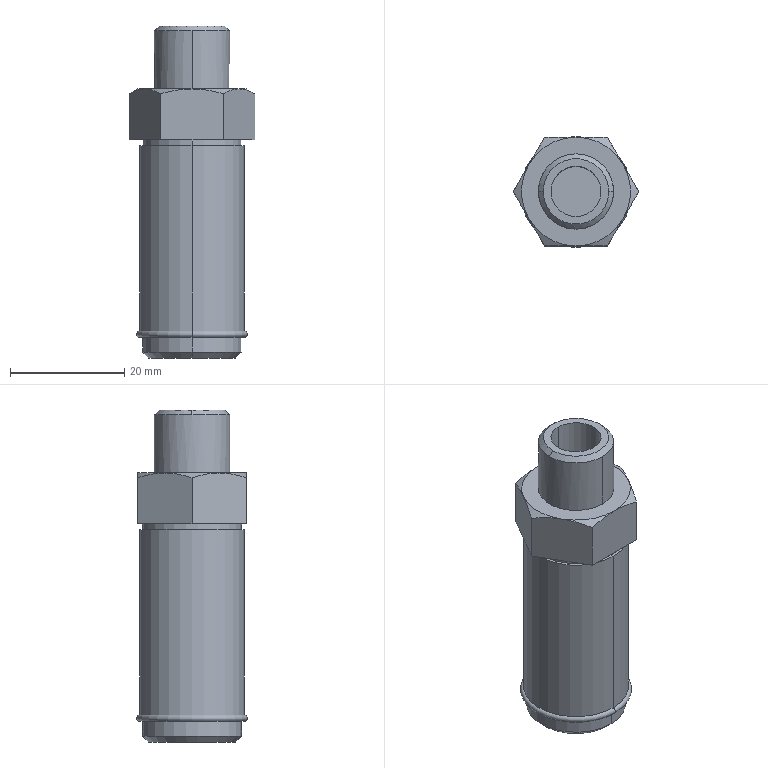Part | STEP file | _HSV08 Body.... | 1 solid | 40 faces | box 21.939 x 19.4 x 58 mm | volume 11796 mm3 | plane 14 | cylinder 12 | cone 12 | torus 2 | commonest cylinder face diameters 17.3 x4 8.771 x2 11.445 x2 13.157 x2 18.3 x2
STEP:
#1=CARTESIAN_POINT('',(0.,-9.15,1.1));
#2=VERTEX_POINT('',#1);
#3=CARTESIAN_POINT('',(0.,9.15,1.1));
#4=VERTEX_POINT('',#3);
#5=CARTESIAN_POINT('',(0.,0.,1.1));
#6=DIRECTION('',(0.,0.,1.));
#7=DIRECTION('',(0.,-1.,0.));
#8=AXIS2_PLACEMENT_3D('',#5,#6,#7);
#9=CIRCLE('',#8,9.15);
#10=EDGE_CURVE('',#2,#4,#9,.T.);
#11=ORIENTED_EDGE('',*,*,#10,.T.);
#12=CARTESIAN_POINT('',(0.,9.15,33.5));
#13=VERTEX_POINT('',#12);
#14=CARTESIAN_POINT('',(0.,9.15,-3.6));
#15=DIRECTION('',(0.,0.,1.));
#16=VECTOR('',#15,1000.);
#17=LINE('',#14,#16);
#18=EDGE_CURVE('',#4,#13,#17,.T.);
#19=ORIENTED_EDGE('',*,*,#18,.T.);
#20=CARTESIAN_POINT('',(0.,-9.15,33.5));
#21=VERTEX_POINT('',#20);
#22=CARTESIAN_POINT('',(0.,0.,33.5));
#23=DIRECTION('',(0.,0.,-1.));
#24=DIRECTION('',(0.,-1.,0.));
#25=AXIS2_PLACEMENT_3D('',#22,#23,#24);
#26=CIRCLE('',#25,9.15);
#27=EDGE_CURVE('',#13,#21,#26,.T.);
#28=ORIENTED_EDGE('',*,*,#27,.T.);
#29=CARTESIAN_POINT('',(0.,-9.15,-3.6));
#30=DIRECTION('',(0.,0.,1.));
#31=VECTOR('',#30,1000.);
#32=LINE('',#29,#31);
#33=EDGE_CURVE('',#2,#21,#32,.T.);
#34=ORIENTED_EDGE('',*,*,#33,.F.);
#35=EDGE_LOOP('',(#11,#19,#28,#34));
#36=FACE_OUTER_BOUND('',#35,.T.);
#37=CARTESIAN_POINT('',(0.,0.,-3.6));
#38=DIRECTION('',(0.,0.,1.));
#39=DIRECTION('',(0.,-1.,0.));
#40=AXIS2_PLACEMENT_3D('',#37,#38,#39);
#41=CYLINDRICAL_SURFACE('',#40,9.15);
#42=ADVANCED_FACE('',(#36),#41,.T.);
#43=ORIENTED_EDGE('',*,*,#10,.F.);
#44=CARTESIAN_POINT('',(0.,-9.15,0.));
#45=VERTEX_POINT('',#44);
#46=CARTESIAN_POINT('',(0.,-9.15,0.55));
#47=DIRECTION('',(1.,0.,0.));
#48=DIRECTION('',(0.,1.,0.));
#49=AXIS2_PLACEMENT_3D('',#46,#47,#48);
#50=CIRCLE('',#49,0.55);
#51=EDGE_CURVE('',#2,#45,#50,.T.);
#52=ORIENTED_EDGE('',*,*,#51,.T.);
#53=CARTESIAN_POINT('',(0.,9.15,0.));
#54=VERTEX_POINT('',#53);
#55=CARTESIAN_POINT('',(0.,0.,0.));
#56=DIRECTION('',(0.,0.,1.));
#57=DIRECTION('',(0.,1.,0.));
#58=AXIS2_PLACEMENT_3D('',#55,#56,#57);
#59=CIRCLE('',#58,9.15);
#60=EDGE_CURVE('',#45,#54,#59,.T.);
#61=ORIENTED_EDGE('',*,*,#60,.T.);
#62=CARTESIAN_POINT('',(0.,9.15,0.55));
#63=DIRECTION('',(-1.,0.,0.));
#64=DIRECTION('',(0.,0.,1.));
#65=AXIS2_PLACEMENT_3D('',#62,#63,#64);
#66=CIRCLE('',#65,0.55);
#67=EDGE_CURVE('',#4,#54,#66,.T.);
#68=ORIENTED_EDGE('',*,*,#67,.F.);
#69=EDGE_LOOP('',(#43,#52,#61,#68));
#70=FACE_OUTER_BOUND('',#69,.T.);
#71=CARTESIAN_POINT('',(0.,0.,0.55));
#72=DIRECTION('',(0.,0.,-1.));
#73=DIRECTION('',(0.,1.,0.));
#74=AXIS2_PLACEMENT_3D('',#71,#72,#73);
#75=TOROIDAL_SURFACE('',#74,9.15,0.55);
#76=ADVANCED_FACE('',(#70),#75,.T.);
#77=CARTESIAN_POINT('',(0.,-8.65,33.5));
#78=VERTEX_POINT('',#77);
#79=CARTESIAN_POINT('',(0.,8.65,33.5));
#80=VERTEX_POINT('',#79);
#81=CARTESIAN_POINT('',(0.,0.,33.5));
#82=DIRECTION('',(0.,0.,1.));
#83=DIRECTION('',(0.,-1.,0.));
#84=AXIS2_PLACEMENT_3D('',#81,#82,#83);
#85=CIRCLE('',#84,8.65);
#86=EDGE_CURVE('',#78,#80,#85,.T.);
#87=ORIENTED_EDGE('',*,*,#86,.T.);
#88=CARTESIAN_POINT('',(0.,8.65,34.5));
#89=VERTEX_POINT('',#88);
#90=CARTESIAN_POINT('',(0.,8.65,-3.6));
#91=DIRECTION('',(0.,0.,1.));
#92=VECTOR('',#91,1000.);
#93=LINE('',#90,#92);
#94=EDGE_CURVE('',#80,#89,#93,.T.);
#95=ORIENTED_EDGE('',*,*,#94,.T.);
#96=CARTESIAN_POINT('',(0.,-8.65,34.5));
#97=VERTEX_POINT('',#96);
#98=CARTESIAN_POINT('',(0.,0.,34.5));
#99=DIRECTION('',(0.,0.,-1.));
#100=DIRECTION('',(0.,-1.,0.));
#101=AXIS2_PLACEMENT_3D('',#98,#99,#100);
#102=CIRCLE('',#101,8.65);
#103=EDGE_CURVE('',#89,#97,#102,.T.);
#104=ORIENTED_EDGE('',*,*,#103,.T.);
#105=CARTESIAN_POINT('',(0.,-8.65,-3.6));
#106=DIRECTION('',(0.,0.,1.));
#107=VECTOR('',#106,1000.);
#108=LINE('',#105,#107);
#109=EDGE_CURVE('',#78,#97,#108,.T.);
#110=ORIENTED_EDGE('',*,*,#109,.F.);
#111=EDGE_LOOP('',(#87,#95,#104,#110));
#112=FACE_OUTER_BOUND('',#111,.T.);
#113=CARTESIAN_POINT('',(0.,0.,-3.6));
#114=DIRECTION('',(0.,0.,1.));
#115=DIRECTION('',(0.,-1.,0.));
#116=AXIS2_PLACEMENT_3D('',#113,#114,#115);
#117=CYLINDRICAL_SURFACE('',#116,8.65);
#118=ADVANCED_FACE('',(#112),#117,.T.);
#119=CARTESIAN_POINT('',(0.,-8.65,-2.6));
#120=VERTEX_POINT('',#119);
#121=CARTESIAN_POINT('',(0.,8.65,-2.6));
#122=VERTEX_POINT('',#121);
#123=CARTESIAN_POINT('',(0.,0.,-2.6));
#124=DIRECTION('',(0.,0.,1.));
#125=DIRECTION('',(0.,-1.,0.));
#126=AXIS2_PLACEMENT_3D('',#123,#124,#125);
#127=CIRCLE('',#126,8.65);
#128=EDGE_CURVE('',#120,#122,#127,.T.);
#129=ORIENTED_EDGE('',*,*,#128,.T.);
#130=CARTESIAN_POINT('',(0.,8.65,0.));
#131=VERTEX_POINT('',#130);
#132=CARTESIAN_POINT('',(0.,8.65,-3.6));
#133=DIRECTION('',(0.,0.,1.));
#134=VECTOR('',#133,1000.);
#135=LINE('',#132,#134);
#136=EDGE_CURVE('',#122,#131,#135,.T.);
#137=ORIENTED_EDGE('',*,*,#136,.T.);
#138=CARTESIAN_POINT('',(0.,-8.65,0.));
#139=VERTEX_POINT('',#138);
#140=CARTESIAN_POINT('',(0.,0.,0.));
#141=DIRECTION('',(0.,0.,-1.));
#142=DIRECTION('',(0.,-1.,0.));
#143=AXIS2_PLACEMENT_3D('',#140,#141,#142);
#144=CIRCLE('',#143,8.65);
#145=EDGE_CURVE('',#131,#139,#144,.T.);
#146=ORIENTED_EDGE('',*,*,#145,.T.);
#147=CARTESIAN_POINT('',(0.,-8.65,-3.6));
#148=DIRECTION('',(0.,0.,1.));
#149=VECTOR('',#148,1000.);
#150=LINE('',#147,#149);
#151=EDGE_CURVE('',#120,#139,#150,.T.);
#152=ORIENTED_EDGE('',*,*,#151,.F.);
#153=EDGE_LOOP('',(#129,#137,#146,#152));
#154=FACE_OUTER_BOUND('',#153,.T.);
#155=CARTESIAN_POINT('',(0.,0.,-3.6));
#156=DIRECTION('',(0.,0.,1.));
#157=DIRECTION('',(0.,-1.,0.));
#158=AXIS2_PLACEMENT_3D('',#155,#156,#157);
#159=CYLINDRICAL_SURFACE('',#158,8.65);
#160=ADVANCED_FACE('',(#154),#159,.T.);
#161=CARTESIAN_POINT('',(0.,-7.65,-3.6));
#162=VERTEX_POINT('',#161);
#163=CARTESIAN_POINT('',(0.,7.65,-3.6));
#164=VERTEX_POINT('',#163);
#165=CARTESIAN_POINT('',(0.,0.,-3.6));
#166=DIRECTION('',(0.,0.,1.));
#167=DIRECTION('',(0.,-1.,0.));
#168=AXIS2_PLACEMENT_3D('',#165,#166,#167);
#169=CIRCLE('',#168,7.65);
#170=EDGE_CURVE('',#162,#164,#169,.T.);
#171=ORIENTED_EDGE('',*,*,#170,.T.);
#172=CARTESIAN_POINT('',(0.,8.65,-2.6));
#173=DIRECTION('',(0.,0.7071,0.7071));
#174=VECTOR('',#173,1000.);
#175=LINE('',#172,#174);
#176=EDGE_CURVE('',#164,#122,#175,.T.);
#177=ORIENTED_EDGE('',*,*,#176,.T.);
#178=ORIENTED_EDGE('',*,*,#128,.F.);
#179=CARTESIAN_POINT('',(0.,-8.65,-2.6));
#180=DIRECTION('',(0.,-0.7071,0.7071));
#181=VECTOR('',#180,1000.);
#182=LINE('',#179,#181);
#183=EDGE_CURVE('',#162,#120,#182,.T.);
#184=ORIENTED_EDGE('',*,*,#183,.F.);
#185=EDGE_LOOP('',(#171,#177,#178,#184));
#186=FACE_OUTER_BOUND('',#185,.T.);
#187=CARTESIAN_POINT('',(0.,0.,-2.6));
#188=DIRECTION('',(0.,0.,1.));
#189=DIRECTION('',(0.,-1.,0.));
#190=AXIS2_PLACEMENT_3D('',#187,#188,#189);
#191=CONICAL_SURFACE('',#190,8.65,0.7854);
#192=ADVANCED_FACE('',(#186),#191,.T.);
#193=CARTESIAN_POINT('',(0.,-6.578,43.4));
#194=VERTEX_POINT('',#193);
#195=CARTESIAN_POINT('',(0.,6.578,43.4));
#196=VERTEX_POINT('',#195);
#197=CARTESIAN_POINT('',(0.,0.,43.4));
#198=DIRECTION('',(0.,0.,1.));
#199=DIRECTION('',(0.,-1.,0.));
#200=AXIS2_PLACEMENT_3D('',#197,#198,#199);
#201=CIRCLE('',#200,6.578);
#202=EDGE_CURVE('',#194,#196,#201,.T.);
#203=ORIENTED_EDGE('',*,*,#202,.T.);
#204=CARTESIAN_POINT('',(0.,6.579,53.544));
#205=VERTEX_POINT('',#204);
#206=CARTESIAN_POINT('',(0.,6.578,-3.6));
#207=DIRECTION('',(0.,0.,1.));
#208=VECTOR('',#207,1000.);
#209=LINE('',#206,#208);
#210=EDGE_CURVE('',#196,#205,#209,.T.);
#211=ORIENTED_EDGE('',*,*,#210,.T.);
#212=CARTESIAN_POINT('',(6.579,0.,53.544));
#213=VERTEX_POINT('',#212);
#214=CARTESIAN_POINT('',(0.,0.,53.544));
#215=DIRECTION('',(0.,0.,-1.));
#216=DIRECTION('',(0.,-1.,0.));
#217=AXIS2_PLACEMENT_3D('',#214,#215,#216);
#218=CIRCLE('',#217,6.578);
#219=EDGE_CURVE('',#205,#213,#218,.T.);
#220=ORIENTED_EDGE('',*,*,#219,.T.);
#221=CARTESIAN_POINT('',(0.,-6.578,53.544));
#222=VERTEX_POINT('',#221);
#223=CARTESIAN_POINT('',(0.,0.,53.544));
#224=DIRECTION('',(0.,0.,-1.));
#225=DIRECTION('',(0.,-1.,0.));
#226=AXIS2_PLACEMENT_3D('',#223,#224,#225);
#227=CIRCLE('',#226,6.578);
#228=EDGE_CURVE('',#213,#222,#227,.T.);
#229=ORIENTED_EDGE('',*,*,#228,.T.);
#230=CARTESIAN_POINT('',(0.,-6.578,-3.6));
#231=DIRECTION('',(0.,0.,1.));
#232=VECTOR('',#231,1000.);
#233=LINE('',#230,#232);
#234=EDGE_CURVE('',#194,#222,#233,.T.);
#235=ORIENTED_EDGE('',*,*,#234,.F.);
#236=EDGE_LOOP('',(#203,#211,#220,#229,#235));
#237=FACE_OUTER_BOUND('',#236,.T.);
#238=CARTESIAN_POINT('',(0.,0.,-3.6));
#239=DIRECTION('',(0.,0.,1.));
#240=DIRECTION('',(0.,-1.,0.));
#241=AXIS2_PLACEMENT_3D('',#238,#239,#240);
#242=CYLINDRICAL_SURFACE('',#241,6.578);
#243=ADVANCED_FACE('',(#237),#242,.T.);
#244=CARTESIAN_POINT('',(0.,-5.722,-2.744));
#245=VERTEX_POINT('',#244);
#246=CARTESIAN_POINT('',(0.,5.722,-2.744));
#247=VERTEX_POINT('',#246);
#248=CARTESIAN_POINT('',(0.,0.,-2.744));
#249=DIRECTION('',(0.,0.,-1.));
#250=DIRECTION('',(0.,1.,0.));
#251=AXIS2_PLACEMENT_3D('',#248,#249,#250);
#252=CIRCLE('',#251,5.722);
#253=EDGE_CURVE('',#245,#247,#252,.T.);
#254=ORIENTED_EDGE('',*,*,#253,.F.);
#255=CARTESIAN_POINT('',(0.,-6.578,-3.6));
#256=VERTEX_POINT('',#255);
#257=CARTESIAN_POINT('',(0.,-6.579,-3.6));
#258=DIRECTION('',(0.,-0.7071,-0.7071));
#259=VECTOR('',#258,1000.);
#260=LINE('',#257,#259);
#261=EDGE_CURVE('',#245,#256,#260,.T.);
#262=ORIENTED_EDGE('',*,*,#261,.T.);
#263=CARTESIAN_POINT('',(0.,6.578,-3.6));
#264=VERTEX_POINT('',#263);
#265=CARTESIAN_POINT('',(0.,0.,-3.6));
#266=DIRECTION('',(0.,0.,-1.));
#267=DIRECTION('',(0.,1.,0.));
#268=AXIS2_PLACEMENT_3D('',#265,#266,#267);
#269=CIRCLE('',#268,6.578);
#270=EDGE_CURVE('',#256,#264,#269,.T.);
#271=ORIENTED_EDGE('',*,*,#270,.T.);
#272=CARTESIAN_POINT('',(0.,6.579,-3.6));
#273=DIRECTION('',(0.,0.7071,-0.7071));
#274=VECTOR('',#273,1000.);
#275=LINE('',#272,#274);
#276=EDGE_CURVE('',#247,#264,#275,.T.);
#277=ORIENTED_EDGE('',*,*,#276,.F.);
#278=EDGE_LOOP('',(#254,#262,#271,#277));
#279=FACE_OUTER_BOUND('',#278,.T.);
#280=CARTESIAN_POINT('',(0.,0.,-3.6));
#281=DIRECTION('',(0.,0.,-1.));
#282=DIRECTION('',(0.,1.,0.));
#283=AXIS2_PLACEMENT_3D('',#280,#281,#282);
#284=CONICAL_SURFACE('',#283,6.579,0.7854);
#285=ADVANCED_FACE('',(#279),#284,.F.);
#286=CARTESIAN_POINT('',(-5.722,0.,54.4));
#287=VERTEX_POINT('',#286);
#288=CARTESIAN_POINT('',(5.722,0.,54.4));
#289=VERTEX_POINT('',#288);
#290=CARTESIAN_POINT('',(0.,0.,54.4));
#291=DIRECTION('',(0.,0.,-1.));
#292=DIRECTION('',(-1.,0.,0.));
#293=AXIS2_PLACEMENT_3D('',#290,#291,#292);
#294=CIRCLE('',#293,5.722);
#295=EDGE_CURVE('',#287,#289,#294,.T.);
#296=ORIENTED_EDGE('',*,*,#295,.T.);
#297=CARTESIAN_POINT('',(6.578,0.,53.544));
#298=DIRECTION('',(0.7071,0.,-0.7071));
#299=VECTOR('',#298,1000.);
#300=LINE('',#297,#299);
#301=EDGE_CURVE('',#289,#213,#300,.T.);
#302=ORIENTED_EDGE('',*,*,#301,.T.);
#303=ORIENTED_EDGE('',*,*,#219,.F.);
#304=CARTESIAN_POINT('',(-6.579,0.,53.544));
#305=VERTEX_POINT('',#304);
#306=CARTESIAN_POINT('',(0.,0.,53.544));
#307=DIRECTION('',(0.,0.,-1.));
#308=DIRECTION('',(0.,-1.,0.));
#309=AXIS2_PLACEMENT_3D('',#306,#307,#308);
#310=CIRCLE('',#309,6.578);
#311=EDGE_CURVE('',#305,#205,#310,.T.);
#312=ORIENTED_EDGE('',*,*,#311,.F.);
#313=CARTESIAN_POINT('',(-6.578,0.,53.544));
#314=DIRECTION('',(-0.7071,0.,-0.7071));
#315=VECTOR('',#314,1000.);
#316=LINE('',#313,#315);
#317=EDGE_CURVE('',#287,#305,#316,.T.);
#318=ORIENTED_EDGE('',*,*,#317,.F.);
#319=EDGE_LOOP('',(#296,#302,#303,#312,#318));
#320=FACE_OUTER_BOUND('',#319,.T.);
#321=CARTESIAN_POINT('',(0.,0.,53.544));
#322=DIRECTION('',(0.,0.,-1.));
#323=DIRECTION('',(-1.,0.,0.));
#324=AXIS2_PLACEMENT_3D('',#321,#322,#323);
#325=CONICAL_SURFACE('',#324,6.578,0.7854);
#326=ADVANCED_FACE('',(#320),#325,.T.);
#327=ORIENTED_EDGE('',*,*,#253,.T.);
#328=CARTESIAN_POINT('',(0.,5.723,7.4));
#329=VERTEX_POINT('',#328);
#330=CARTESIAN_POINT('',(0.,5.723,-3.6));
#331=DIRECTION('',(0.,0.,1.));
#332=VECTOR('',#331,1000.);
#333=LINE('',#330,#332);
#334=EDGE_CURVE('',#247,#329,#333,.T.);
#335=ORIENTED_EDGE('',*,*,#334,.T.);
#336=CARTESIAN_POINT('',(0.,-5.723,7.4));
#337=VERTEX_POINT('',#336);
#338=CARTESIAN_POINT('',(0.,0.,7.4));
#339=DIRECTION('',(0.,0.,-1.));
#340=DIRECTION('',(0.,-1.,0.));
#341=AXIS2_PLACEMENT_3D('',#338,#339,#340);
#342=CIRCLE('',#341,5.723);
#343=EDGE_CURVE('',#337,#329,#342,.T.);
#344=ORIENTED_EDGE('',*,*,#343,.F.);
#345=CARTESIAN_POINT('',(0.,-5.723,-3.6));
#346=DIRECTION('',(0.,0.,1.));
#347=VECTOR('',#346,1000.);
#348=LINE('',#345,#347);
#349=EDGE_CURVE('',#245,#337,#348,.T.);
#350=ORIENTED_EDGE('',*,*,#349,.F.);
#351=EDGE_LOOP('',(#327,#335,#344,#350));
#352=FACE_OUTER_BOUND('',#351,.T.);
#353=CARTESIAN_POINT('',(0.,0.,-3.6));
#354=DIRECTION('',(0.,0.,1.));
#355=DIRECTION('',(0.,-1.,0.));
#356=AXIS2_PLACEMENT_3D('',#353,#354,#355);
#357=CYLINDRICAL_SURFACE('',#356,5.723);
#358=ADVANCED_FACE('',(#352),#357,.F.);
#359=CARTESIAN_POINT('',(0.,4.386,34.4));
#360=VERTEX_POINT('',#359);
#361=CARTESIAN_POINT('',(0.,-4.386,34.4));
#362=VERTEX_POINT('',#361);
#363=CARTESIAN_POINT('',(0.,0.,34.4));
#364=DIRECTION('',(0.,0.,1.));
#365=DIRECTION('',(0.,-1.,0.));
#366=AXIS2_PLACEMENT_3D('',#363,#364,#365);
#367=CIRCLE('',#366,4.386);
#368=EDGE_CURVE('',#360,#362,#367,.T.);
#369=ORIENTED_EDGE('',*,*,#368,.F.);
#370=CARTESIAN_POINT('',(0.,4.386,54.4));
#371=VERTEX_POINT('',#370);
#372=CARTESIAN_POINT('',(0.,4.386,-3.6));
#373=DIRECTION('',(0.,0.,1.));
#374=VECTOR('',#373,1000.);
#375=LINE('',#372,#374);
#376=EDGE_CURVE('',#360,#371,#375,.T.);
#377=ORIENTED_EDGE('',*,*,#376,.T.);
#378=CARTESIAN_POINT('',(0.,-4.386,54.4));
#379=VERTEX_POINT('',#378);
#380=CARTESIAN_POINT('',(0.,0.,54.4));
#381=DIRECTION('',(0.,0.,1.));
#382=DIRECTION('',(0.,-1.,0.));
#383=AXIS2_PLACEMENT_3D('',#380,#381,#382);
#384=CIRCLE('',#383,4.386);
#385=EDGE_CURVE('',#371,#379,#384,.T.);
#386=ORIENTED_EDGE('',*,*,#385,.T.);
#387=CARTESIAN_POINT('',(0.,-4.386,-3.6));
#388=DIRECTION('',(0.,0.,1.));
#389=VECTOR('',#388,1000.);
#390=LINE('',#387,#389);
#391=EDGE_CURVE('',#362,#379,#390,.T.);
#392=ORIENTED_EDGE('',*,*,#391,.F.);
#393=EDGE_LOOP('',(#369,#377,#386,#392));
#394=FACE_OUTER_BOUND('',#393,.T.);
#395=CARTESIAN_POINT('',(0.,0.,-3.6));
#396=DIRECTION('',(0.,0.,1.));
#397=DIRECTION('',(0.,-1.,0.));
#398=AXIS2_PLACEMENT_3D('',#395,#396,#397);
#399=CYLINDRICAL_SURFACE('',#398,4.386);
#400=ADVANCED_FACE('',(#394),#399,.F.);
#401=ORIENTED_EDGE('',*,*,#18,.F.);
#402=CARTESIAN_POINT('',(0.,0.,1.1));
#403=DIRECTION('',(0.,0.,1.));
#404=DIRECTION('',(0.,-1.,0.));
#405=AXIS2_PLACEMENT_3D('',#402,#403,#404);
#406=CIRCLE('',#405,9.15);
#407=EDGE_CURVE('',#4,#2,#406,.T.);
#408=ORIENTED_EDGE('',*,*,#407,.T.);
#409=ORIENTED_EDGE('',*,*,#33,.T.);
#410=CARTESIAN_POINT('',(0.,0.,33.5));
#411=DIRECTION('',(0.,0.,-1.));
#412=DIRECTION('',(0.,-1.,0.));
#413=AXIS2_PLACEMENT_3D('',#410,#411,#412);
#414=CIRCLE('',#413,9.15);
#415=EDGE_CURVE('',#21,#13,#414,.T.);
#416=ORIENTED_EDGE('',*,*,#415,.T.);
#417=EDGE_LOOP('',(#401,#408,#409,#416));
#418=FACE_OUTER_BOUND('',#417,.T.);
#419=CARTESIAN_POINT('',(0.,0.,-3.6));
#420=DIRECTION('',(0.,0.,1.));
#421=DIRECTION('',(0.,-1.,0.));
#422=AXIS2_PLACEMENT_3D('',#419,#420,#421);
#423=CYLINDRICAL_SURFACE('',#422,9.15);
#424=ADVANCED_FACE('',(#418),#423,.T.);
#425=ORIENTED_EDGE('',*,*,#415,.F.);
#426=ORIENTED_EDGE('',*,*,#27,.F.);
#427=EDGE_LOOP('',(#425,#426));
#428=FACE_OUTER_BOUND('',#427,.T.);
#429=ORIENTED_EDGE('',*,*,#86,.F.);
#430=CARTESIAN_POINT('',(0.,0.,33.5));
#431=DIRECTION('',(0.,0.,1.));
#432=DIRECTION('',(0.,-1.,0.));
#433=AXIS2_PLACEMENT_3D('',#430,#431,#432);
#434=CIRCLE('',#433,8.65);
#435=EDGE_CURVE('',#80,#78,#434,.T.);
#436=ORIENTED_EDGE('',*,*,#435,.F.);
#437=EDGE_LOOP('',(#429,#436));
#438=FACE_BOUND('',#437,.T.);
#439=CARTESIAN_POINT('',(0.,8.65,33.5));
#440=DIRECTION('',(0.,0.,-1.));
#441=DIRECTION('',(0.,1.,0.));
#442=AXIS2_PLACEMENT_3D('',#439,#440,#441);
#443=PLANE('',#442);
#444=ADVANCED_FACE('',(#428,#438),#443,.F.);
#445=ORIENTED_EDGE('',*,*,#51,.F.);
#446=ORIENTED_EDGE('',*,*,#407,.F.);
#447=ORIENTED_EDGE('',*,*,#67,.T.);
#448=CARTESIAN_POINT('',(0.,0.,0.));
#449=DIRECTION('',(0.,0.,1.));
#450=DIRECTION('',(0.,1.,0.));
#451=AXIS2_PLACEMENT_3D('',#448,#449,#450);
#452=CIRCLE('',#451,9.15);
#453=EDGE_CURVE('',#54,#45,#452,.T.);
#454=ORIENTED_EDGE('',*,*,#453,.T.);
#455=EDGE_LOOP('',(#445,#446,#447,#454));
#456=FACE_OUTER_BOUND('',#455,.T.);
#457=CARTESIAN_POINT('',(0.,0.,0.55));
#458=DIRECTION('',(0.,0.,-1.));
#459=DIRECTION('',(0.,1.,0.));
#460=AXIS2_PLACEMENT_3D('',#457,#458,#459);
#461=TOROIDAL_SURFACE('',#460,9.15,0.55);
#462=ADVANCED_FACE('',(#456),#461,.T.);
#463=ORIENTED_EDGE('',*,*,#94,.F.);
#464=ORIENTED_EDGE('',*,*,#435,.T.);
#465=ORIENTED_EDGE('',*,*,#109,.T.);
#466=CARTESIAN_POINT('',(0.,0.,34.5));
#467=DIRECTION('',(0.,0.,-1.));
#468=DIRECTION('',(0.,-1.,0.));
#469=AXIS2_PLACEMENT_3D('',#466,#467,#468);
#470=CIRCLE('',#469,8.65);
#471=EDGE_CURVE('',#97,#89,#470,.T.);
#472=ORIENTED_EDGE('',*,*,#471,.T.);
#473=EDGE_LOOP('',(#463,#464,#465,#472));
#474=FACE_OUTER_BOUND('',#473,.T.);
#475=CARTESIAN_POINT('',(0.,0.,-3.6));
#476=DIRECTION('',(0.,0.,1.));
#477=DIRECTION('',(0.,-1.,0.));
#478=AXIS2_PLACEMENT_3D('',#475,#476,#477);
#479=CYLINDRICAL_SURFACE('',#478,8.65);
#480=ADVANCED_FACE('',(#474),#479,.T.);
#481=ORIENTED_EDGE('',*,*,#471,.F.);
#482=ORIENTED_EDGE('',*,*,#103,.F.);
#483=EDGE_LOOP('',(#481,#482));
#484=FACE_BOUND('',#483,.T.);
#485=CARTESIAN_POINT('',(5.485,9.5,34.5));
#486=VERTEX_POINT('',#485);
#487=CARTESIAN_POINT('',(-5.485,9.5,34.5));
#488=VERTEX_POINT('',#487);
#489=CARTESIAN_POINT('',(0.,9.5,34.5));
#490=DIRECTION('',(-1.,0.,0.));
#491=VECTOR('',#490,1000.);
#492=LINE('',#489,#491);
#493=EDGE_CURVE('',#486,#488,#492,.T.);
#494=ORIENTED_EDGE('',*,*,#493,.F.);
#495=CARTESIAN_POINT('',(10.97,0.,34.5));
#496=VERTEX_POINT('',#495);
#497=CARTESIAN_POINT('',(10.97,0.,34.5));
#498=DIRECTION('',(-0.5,0.866,0.));
#499=VECTOR('',#498,1000.);
#500=LINE('',#497,#499);
#501=EDGE_CURVE('',#496,#486,#500,.T.);
#502=ORIENTED_EDGE('',*,*,#501,.F.);
#503=CARTESIAN_POINT('',(5.485,-9.5,34.5));
#504=VERTEX_POINT('',#503);
#505=CARTESIAN_POINT('',(5.485,-9.5,34.5));
#506=DIRECTION('',(0.5,0.866,0.));
#507=VECTOR('',#506,1000.);
#508=LINE('',#505,#507);
#509=EDGE_CURVE('',#504,#496,#508,.T.);
#510=ORIENTED_EDGE('',*,*,#509,.F.);
#511=CARTESIAN_POINT('',(-5.485,-9.5,34.5));
#512=VERTEX_POINT('',#511);
#513=CARTESIAN_POINT('',(0.,-9.5,34.5));
#514=DIRECTION('',(1.,0.,0.));
#515=VECTOR('',#514,1000.);
#516=LINE('',#513,#515);
#517=EDGE_CURVE('',#512,#504,#516,.T.);
#518=ORIENTED_EDGE('',*,*,#517,.F.);
#519=CARTESIAN_POINT('',(-10.97,0.,34.5));
#520=VERTEX_POINT('',#519);
#521=CARTESIAN_POINT('',(-10.97,0.,34.5));
#522=DIRECTION('',(0.5,-0.866,0.));
#523=VECTOR('',#522,1000.);
#524=LINE('',#521,#523);
#525=EDGE_CURVE('',#520,#512,#524,.T.);
#526=ORIENTED_EDGE('',*,*,#525,.F.);
#527=CARTESIAN_POINT('',(-5.485,9.5,34.5));
#528=DIRECTION('',(-0.5,-0.866,0.));
#529=VECTOR('',#528,1000.);
#530=LINE('',#527,#529);
#531=EDGE_CURVE('',#488,#520,#530,.T.);
#532=ORIENTED_EDGE('',*,*,#531,.F.);
#533=EDGE_LOOP('',(#494,#502,#510,#518,#526,#532));
#534=FACE_OUTER_BOUND('',#533,.T.);
#535=CARTESIAN_POINT('',(0.,19.,34.5));
#536=DIRECTION('',(0.,0.,1.));
#537=DIRECTION('',(0.,-1.,0.));
#538=AXIS2_PLACEMENT_3D('',#535,#536,#537);
#539=PLANE('',#538);
#540=ADVANCED_FACE('',(#484,#534),#539,.F.);
#541=CARTESIAN_POINT('',(0.,0.,0.));
#542=DIRECTION('',(0.,0.,-1.));
#543=DIRECTION('',(0.,-1.,0.));
#544=AXIS2_PLACEMENT_3D('',#541,#542,#543);
#545=CIRCLE('',#544,8.65);
#546=EDGE_CURVE('',#139,#131,#545,.T.);
#547=ORIENTED_EDGE('',*,*,#546,.F.);
#548=ORIENTED_EDGE('',*,*,#145,.F.);
#549=EDGE_LOOP('',(#547,#548));
#550=FACE_BOUND('',#549,.T.);
#551=ORIENTED_EDGE('',*,*,#453,.F.);
#552=ORIENTED_EDGE('',*,*,#60,.F.);
#553=EDGE_LOOP('',(#551,#552));
#554=FACE_OUTER_BOUND('',#553,.T.);
#555=CARTESIAN_POINT('',(0.,9.15,0.));
#556=DIRECTION('',(0.,0.,1.));
#557=DIRECTION('',(0.,-1.,0.));
#558=AXIS2_PLACEMENT_3D('',#555,#556,#557);
#559=PLANE('',#558);
#560=ADVANCED_FACE('',(#550,#554),#559,.F.);
#561=CARTESIAN_POINT('',(-8.227,4.75,43.4));
#562=VERTEX_POINT('',#561);
#563=CARTESIAN_POINT('',(-5.485,9.5,42.551));
#564=VERTEX_POINT('',#563);
#565=CARTESIAN_POINT('',(-8.227,4.75,43.4));
#566=CARTESIAN_POINT('',(-7.759,5.561,43.4));
#567=CARTESIAN_POINT('',(-7.298,6.36,43.319));
#568=CARTESIAN_POINT('',(-6.384,7.942,43.023));
#569=CARTESIAN_POINT('',(-5.933,8.724,42.81));
#570=CARTESIAN_POINT('',(-5.485,9.5,42.551));
#571=B_SPLINE_CURVE_WITH_KNOTS('',3,(#565,#566,#567,#568,#569,#570),.UNSPECIFIED.,.F.,.F.,(4,2,4),(0.,0.002775,0.00555),.UNSPECIFIED.);
#572=EDGE_CURVE('',#562,#564,#571,.T.);
#573=ORIENTED_EDGE('',*,*,#572,.T.);
#574=CARTESIAN_POINT('',(-5.485,9.5,34.5));
#575=DIRECTION('',(0.,0.,-1.));
#576=VECTOR('',#575,1000.);
#577=LINE('',#574,#576);
#578=EDGE_CURVE('',#564,#488,#577,.T.);
#579=ORIENTED_EDGE('',*,*,#578,.T.);
#580=ORIENTED_EDGE('',*,*,#531,.T.);
#581=CARTESIAN_POINT('',(-10.97,0.,42.551));
#582=VERTEX_POINT('',#581);
#583=CARTESIAN_POINT('',(-10.97,0.,34.5));
#584=DIRECTION('',(0.,0.,1.));
#585=VECTOR('',#584,1000.);
#586=LINE('',#583,#585);
#587=EDGE_CURVE('',#520,#582,#586,.T.);
#588=ORIENTED_EDGE('',*,*,#587,.T.);
#589=CARTESIAN_POINT('',(-10.97,0.,42.551));
#590=CARTESIAN_POINT('',(-10.522,0.776,42.81));
#591=CARTESIAN_POINT('',(-10.07,1.558,43.023));
#592=CARTESIAN_POINT('',(-9.157,3.14,43.319));
#593=CARTESIAN_POINT('',(-8.695,3.939,43.4));
#594=CARTESIAN_POINT('',(-8.227,4.75,43.4));
#595=B_SPLINE_CURVE_WITH_KNOTS('',3,(#589,#590,#591,#592,#593,#594),.UNSPECIFIED.,.F.,.F.,(4,2,4),(0.,0.002775,0.00555),.UNSPECIFIED.);
#596=EDGE_CURVE('',#582,#562,#595,.T.);
#597=ORIENTED_EDGE('',*,*,#596,.T.);
#598=EDGE_LOOP('',(#573,#579,#580,#588,#597));
#599=FACE_OUTER_BOUND('',#598,.T.);
#600=CARTESIAN_POINT('',(-5.485,9.5,34.5));
#601=DIRECTION('',(-0.866,0.5,0.));
#602=DIRECTION('',(-0.5,-0.866,0.));
#603=AXIS2_PLACEMENT_3D('',#600,#601,#602);
#604=PLANE('',#603);
#605=ADVANCED_FACE('',(#599),#604,.T.);
#606=CARTESIAN_POINT('',(0.,9.5,43.4));
#607=VERTEX_POINT('',#606);
#608=CARTESIAN_POINT('',(5.485,9.5,42.551));
#609=VERTEX_POINT('',#608);
#610=CARTESIAN_POINT('',(0.,9.5,43.4));
#611=CARTESIAN_POINT('',(0.936,9.5,43.4));
#612=CARTESIAN_POINT('',(1.859,9.5,43.319));
#613=CARTESIAN_POINT('',(3.686,9.5,43.023));
#614=CARTESIAN_POINT('',(4.589,9.5,42.81));
#615=CARTESIAN_POINT('',(5.485,9.5,42.551));
#616=B_SPLINE_CURVE_WITH_KNOTS('',3,(#610,#611,#612,#613,#614,#615),.UNSPECIFIED.,.F.,.F.,(4,2,4),(0.,0.002775,0.00555),.UNSPECIFIED.);
#617=EDGE_CURVE('',#607,#609,#616,.T.);
#618=ORIENTED_EDGE('',*,*,#617,.T.);
#619=CARTESIAN_POINT('',(5.485,9.5,34.5));
#620=DIRECTION('',(0.,0.,-1.));
#621=VECTOR('',#620,1000.);
#622=LINE('',#619,#621);
#623=EDGE_CURVE('',#609,#486,#622,.T.);
#624=ORIENTED_EDGE('',*,*,#623,.T.);
#625=ORIENTED_EDGE('',*,*,#493,.T.);
#626=ORIENTED_EDGE('',*,*,#578,.F.);
#627=CARTESIAN_POINT('',(-5.485,9.5,42.551));
#628=CARTESIAN_POINT('',(-4.589,9.5,42.81));
#629=CARTESIAN_POINT('',(-3.686,9.5,43.023));
#630=CARTESIAN_POINT('',(-1.859,9.5,43.319));
#631=CARTESIAN_POINT('',(-0.936,9.5,43.4));
#632=CARTESIAN_POINT('',(0.,9.5,43.4));
#633=B_SPLINE_CURVE_WITH_KNOTS('',3,(#627,#628,#629,#630,#631,#632),.UNSPECIFIED.,.F.,.F.,(4,2,4),(0.,0.002775,0.00555),.UNSPECIFIED.);
#634=EDGE_CURVE('',#564,#607,#633,.T.);
#635=ORIENTED_EDGE('',*,*,#634,.T.);
#636=EDGE_LOOP('',(#618,#624,#625,#626,#635));
#637=FACE_OUTER_BOUND('',#636,.T.);
#638=CARTESIAN_POINT('',(5.485,9.5,34.5));
#639=DIRECTION('',(0.,1.,0.));
#640=DIRECTION('',(0.,0.,1.));
#641=AXIS2_PLACEMENT_3D('',#638,#639,#640);
#642=PLANE('',#641);
#643=ADVANCED_FACE('',(#637),#642,.T.);
#644=CARTESIAN_POINT('',(8.227,4.75,43.4));
#645=VERTEX_POINT('',#644);
#646=CARTESIAN_POINT('',(10.97,0.,42.551));
#647=VERTEX_POINT('',#646);
#648=CARTESIAN_POINT('',(8.227,4.75,43.4));
#649=CARTESIAN_POINT('',(8.695,3.939,43.4));
#650=CARTESIAN_POINT('',(9.157,3.14,43.319));
#651=CARTESIAN_POINT('',(10.07,1.558,43.023));
#652=CARTESIAN_POINT('',(10.522,0.776,42.81));
#653=CARTESIAN_POINT('',(10.97,0.,42.551));
#654=B_SPLINE_CURVE_WITH_KNOTS('',3,(#648,#649,#650,#651,#652,#653),.UNSPECIFIED.,.F.,.F.,(4,2,4),(0.,0.002775,0.00555),.UNSPECIFIED.);
#655=EDGE_CURVE('',#645,#647,#654,.T.);
#656=ORIENTED_EDGE('',*,*,#655,.T.);
#657=CARTESIAN_POINT('',(10.97,0.,34.5));
#658=DIRECTION('',(0.,0.,-1.));
#659=VECTOR('',#658,1000.);
#660=LINE('',#657,#659);
#661=EDGE_CURVE('',#647,#496,#660,.T.);
#662=ORIENTED_EDGE('',*,*,#661,.T.);
#663=ORIENTED_EDGE('',*,*,#501,.T.);
#664=ORIENTED_EDGE('',*,*,#623,.F.);
#665=CARTESIAN_POINT('',(5.485,9.5,42.551));
#666=CARTESIAN_POINT('',(5.933,8.724,42.81));
#667=CARTESIAN_POINT('',(6.384,7.942,43.023));
#668=CARTESIAN_POINT('',(7.298,6.36,43.319));
#669=CARTESIAN_POINT('',(7.759,5.561,43.4));
#670=CARTESIAN_POINT('',(8.227,4.75,43.4));
#671=B_SPLINE_CURVE_WITH_KNOTS('',3,(#665,#666,#667,#668,#669,#670),.UNSPECIFIED.,.F.,.F.,(4,2,4),(0.,0.002775,0.00555),.UNSPECIFIED.);
#672=EDGE_CURVE('',#609,#645,#671,.T.);
#673=ORIENTED_EDGE('',*,*,#672,.T.);
#674=EDGE_LOOP('',(#656,#662,#663,#664,#673));
#675=FACE_OUTER_BOUND('',#674,.T.);
#676=CARTESIAN_POINT('',(10.97,0.,34.5));
#677=DIRECTION('',(0.866,0.5,0.));
#678=DIRECTION('',(-0.5,0.866,0.));
#679=AXIS2_PLACEMENT_3D('',#676,#677,#678);
#680=PLANE('',#679);
#681=ADVANCED_FACE('',(#675),#680,.T.);
#682=CARTESIAN_POINT('',(8.227,-4.75,43.4));
#683=VERTEX_POINT('',#682);
#684=CARTESIAN_POINT('',(5.485,-9.5,42.551));
#685=VERTEX_POINT('',#684);
#686=CARTESIAN_POINT('',(8.227,-4.75,43.4));
#687=CARTESIAN_POINT('',(7.759,-5.561,43.4));
#688=CARTESIAN_POINT('',(7.298,-6.36,43.319));
#689=CARTESIAN_POINT('',(6.384,-7.942,43.023));
#690=CARTESIAN_POINT('',(5.933,-8.724,42.81));
#691=CARTESIAN_POINT('',(5.485,-9.5,42.551));
#692=B_SPLINE_CURVE_WITH_KNOTS('',3,(#686,#687,#688,#689,#690,#691),.UNSPECIFIED.,.F.,.F.,(4,2,4),(0.,0.002775,0.00555),.UNSPECIFIED.);
#693=EDGE_CURVE('',#683,#685,#692,.T.);
#694=ORIENTED_EDGE('',*,*,#693,.T.);
#695=CARTESIAN_POINT('',(5.485,-9.5,34.5));
#696=DIRECTION('',(0.,0.,-1.));
#697=VECTOR('',#696,1000.);
#698=LINE('',#695,#697);
#699=EDGE_CURVE('',#685,#504,#698,.T.);
#700=ORIENTED_EDGE('',*,*,#699,.T.);
#701=ORIENTED_EDGE('',*,*,#509,.T.);
#702=ORIENTED_EDGE('',*,*,#661,.F.);
#703=CARTESIAN_POINT('',(10.97,0.,42.551));
#704=CARTESIAN_POINT('',(10.522,-0.776,42.81));
#705=CARTESIAN_POINT('',(10.07,-1.558,43.023));
#706=CARTESIAN_POINT('',(9.157,-3.14,43.319));
#707=CARTESIAN_POINT('',(8.695,-3.939,43.4));
#708=CARTESIAN_POINT('',(8.227,-4.75,43.4));
#709=B_SPLINE_CURVE_WITH_KNOTS('',3,(#703,#704,#705,#706,#707,#708),.UNSPECIFIED.,.F.,.F.,(4,2,4),(0.,0.002775,0.00555),.UNSPECIFIED.);
#710=EDGE_CURVE('',#647,#683,#709,.T.);
#711=ORIENTED_EDGE('',*,*,#710,.T.);
#712=EDGE_LOOP('',(#694,#700,#701,#702,#711));
#713=FACE_OUTER_BOUND('',#712,.T.);
#714=CARTESIAN_POINT('',(5.485,-9.5,34.5));
#715=DIRECTION('',(0.866,-0.5,0.));
#716=DIRECTION('',(0.5,0.866,0.));
#717=AXIS2_PLACEMENT_3D('',#714,#715,#716);
#718=PLANE('',#717);
#719=ADVANCED_FACE('',(#713),#718,.T.);
#720=CARTESIAN_POINT('',(0.,-9.5,43.4));
#721=VERTEX_POINT('',#720);
#722=CARTESIAN_POINT('',(-5.485,-9.5,42.551));
#723=VERTEX_POINT('',#722);
#724=CARTESIAN_POINT('',(0.,-9.5,43.4));
#725=CARTESIAN_POINT('',(-0.936,-9.5,43.4));
#726=CARTESIAN_POINT('',(-1.859,-9.5,43.319));
#727=CARTESIAN_POINT('',(-3.686,-9.5,43.023));
#728=CARTESIAN_POINT('',(-4.589,-9.5,42.81));
#729=CARTESIAN_POINT('',(-5.485,-9.5,42.551));
#730=B_SPLINE_CURVE_WITH_KNOTS('',3,(#724,#725,#726,#727,#728,#729),.UNSPECIFIED.,.F.,.F.,(4,2,4),(0.,0.002775,0.00555),.UNSPECIFIED.);
#731=EDGE_CURVE('',#721,#723,#730,.T.);
#732=ORIENTED_EDGE('',*,*,#731,.T.);
#733=CARTESIAN_POINT('',(-5.485,-9.5,34.5));
#734=DIRECTION('',(0.,0.,-1.));
#735=VECTOR('',#734,1000.);
#736=LINE('',#733,#735);
#737=EDGE_CURVE('',#723,#512,#736,.T.);
#738=ORIENTED_EDGE('',*,*,#737,.T.);
#739=ORIENTED_EDGE('',*,*,#517,.T.);
#740=ORIENTED_EDGE('',*,*,#699,.F.);
#741=CARTESIAN_POINT('',(5.485,-9.5,42.551));
#742=CARTESIAN_POINT('',(4.589,-9.5,42.81));
#743=CARTESIAN_POINT('',(3.686,-9.5,43.023));
#744=CARTESIAN_POINT('',(1.859,-9.5,43.319));
#745=CARTESIAN_POINT('',(0.936,-9.5,43.4));
#746=CARTESIAN_POINT('',(0.,-9.5,43.4));
#747=B_SPLINE_CURVE_WITH_KNOTS('',3,(#741,#742,#743,#744,#745,#746),.UNSPECIFIED.,.F.,.F.,(4,2,4),(0.,0.002775,0.00555),.UNSPECIFIED.);
#748=EDGE_CURVE('',#685,#721,#747,.T.);
#749=ORIENTED_EDGE('',*,*,#748,.T.);
#750=EDGE_LOOP('',(#732,#738,#739,#740,#749));
#751=FACE_OUTER_BOUND('',#750,.T.);
#752=CARTESIAN_POINT('',(-5.485,-9.5,34.5));
#753=DIRECTION('',(0.,-1.,0.));
#754=DIRECTION('',(0.,0.,-1.));
#755=AXIS2_PLACEMENT_3D('',#752,#753,#754);
#756=PLANE('',#755);
#757=ADVANCED_FACE('',(#751),#756,.T.);
#758=CARTESIAN_POINT('',(-8.227,-4.75,43.4));
#759=VERTEX_POINT('',#758);
#760=CARTESIAN_POINT('',(-8.227,-4.75,43.4));
#761=CARTESIAN_POINT('',(-8.695,-3.939,43.4));
#762=CARTESIAN_POINT('',(-9.157,-3.14,43.319));
#763=CARTESIAN_POINT('',(-10.07,-1.558,43.023));
#764=CARTESIAN_POINT('',(-10.522,-0.776,42.81));
#765=CARTESIAN_POINT('',(-10.97,0.,42.551));
#766=B_SPLINE_CURVE_WITH_KNOTS('',3,(#760,#761,#762,#763,#764,#765),.UNSPECIFIED.,.F.,.F.,(4,2,4),(0.,0.002775,0.00555),.UNSPECIFIED.);
#767=EDGE_CURVE('',#759,#582,#766,.T.);
#768=ORIENTED_EDGE('',*,*,#767,.T.);
#769=ORIENTED_EDGE('',*,*,#587,.F.);
#770=ORIENTED_EDGE('',*,*,#525,.T.);
#771=ORIENTED_EDGE('',*,*,#737,.F.);
#772=CARTESIAN_POINT('',(-5.485,-9.5,42.551));
#773=CARTESIAN_POINT('',(-5.933,-8.724,42.81));
#774=CARTESIAN_POINT('',(-6.384,-7.942,43.023));
#775=CARTESIAN_POINT('',(-7.298,-6.36,43.319));
#776=CARTESIAN_POINT('',(-7.759,-5.561,43.4));
#777=CARTESIAN_POINT('',(-8.227,-4.75,43.4));
#778=B_SPLINE_CURVE_WITH_KNOTS('',3,(#772,#773,#774,#775,#776,#777),.UNSPECIFIED.,.F.,.F.,(4,2,4),(0.,0.002775,0.00555),.UNSPECIFIED.);
#779=EDGE_CURVE('',#723,#759,#778,.T.);
#780=ORIENTED_EDGE('',*,*,#779,.T.);
#781=EDGE_LOOP('',(#768,#769,#770,#771,#780));
#782=FACE_OUTER_BOUND('',#781,.T.);
#783=CARTESIAN_POINT('',(-10.97,0.,34.5));
#784=DIRECTION('',(-0.866,-0.5,0.));
#785=DIRECTION('',(0.5,-0.866,0.));
#786=AXIS2_PLACEMENT_3D('',#783,#784,#785);
#787=PLANE('',#786);
#788=ADVANCED_FACE('',(#782),#787,.T.);
#789=ORIENTED_EDGE('',*,*,#136,.F.);
#790=CARTESIAN_POINT('',(0.,0.,-2.6));
#791=DIRECTION('',(0.,0.,1.));
#792=DIRECTION('',(0.,-1.,0.));
#793=AXIS2_PLACEMENT_3D('',#790,#791,#792);
#794=CIRCLE('',#793,8.65);
#795=EDGE_CURVE('',#122,#120,#794,.T.);
#796=ORIENTED_EDGE('',*,*,#795,.T.);
#797=ORIENTED_EDGE('',*,*,#151,.T.);
#798=ORIENTED_EDGE('',*,*,#546,.T.);
#799=EDGE_LOOP('',(#789,#796,#797,#798));
#800=FACE_OUTER_BOUND('',#799,.T.);
#801=CARTESIAN_POINT('',(0.,0.,-3.6));
#802=DIRECTION('',(0.,0.,1.));
#803=DIRECTION('',(0.,-1.,0.));
#804=AXIS2_PLACEMENT_3D('',#801,#802,#803);
#805=CYLINDRICAL_SURFACE('',#804,8.65);
#806=ADVANCED_FACE('',(#800),#805,.T.);
#807=ORIENTED_EDGE('',*,*,#634,.F.);
#808=ORIENTED_EDGE('',*,*,#572,.F.);
#809=CARTESIAN_POINT('',(0.,0.,43.4));
#810=DIRECTION('',(0.,0.,-1.));
#811=DIRECTION('',(0.,1.,0.));
#812=AXIS2_PLACEMENT_3D('',#809,#810,#811);
#813=CIRCLE('',#812,9.5);
#814=EDGE_CURVE('',#562,#607,#813,.T.);
#815=ORIENTED_EDGE('',*,*,#814,.T.);
#816=EDGE_LOOP('',(#807,#808,#815));
#817=FACE_OUTER_BOUND('',#816,.T.);
#818=CARTESIAN_POINT('',(0.,0.,42.546));
#819=DIRECTION('',(0.,0.,-1.));
#820=DIRECTION('',(0.,1.,0.));
#821=AXIS2_PLACEMENT_3D('',#818,#819,#820);
#822=CONICAL_SURFACE('',#821,10.978,1.047);
#823=ADVANCED_FACE('',(#817),#822,.T.);
#824=ORIENTED_EDGE('',*,*,#596,.F.);
#825=ORIENTED_EDGE('',*,*,#767,.F.);
#826=CARTESIAN_POINT('',(0.,0.,43.4));
#827=DIRECTION('',(0.,0.,-1.));
#828=DIRECTION('',(0.,1.,0.));
#829=AXIS2_PLACEMENT_3D('',#826,#827,#828);
#830=CIRCLE('',#829,9.5);
#831=EDGE_CURVE('',#759,#562,#830,.T.);
#832=ORIENTED_EDGE('',*,*,#831,.T.);
#833=EDGE_LOOP('',(#824,#825,#832));
#834=FACE_OUTER_BOUND('',#833,.T.);
#835=CARTESIAN_POINT('',(0.,0.,42.546));
#836=DIRECTION('',(0.,0.,-1.));
#837=DIRECTION('',(0.,1.,0.));
#838=AXIS2_PLACEMENT_3D('',#835,#836,#837);
#839=CONICAL_SURFACE('',#838,10.978,1.047);
#840=ADVANCED_FACE('',(#834),#839,.T.);
#841=ORIENTED_EDGE('',*,*,#672,.F.);
#842=ORIENTED_EDGE('',*,*,#617,.F.);
#843=CARTESIAN_POINT('',(0.,0.,43.4));
#844=DIRECTION('',(0.,0.,-1.));
#845=DIRECTION('',(-1.,0.,0.));
#846=AXIS2_PLACEMENT_3D('',#843,#844,#845);
#847=CIRCLE('',#846,9.5);
#848=EDGE_CURVE('',#607,#645,#847,.T.);
#849=ORIENTED_EDGE('',*,*,#848,.T.);
#850=EDGE_LOOP('',(#841,#842,#849));
#851=FACE_OUTER_BOUND('',#850,.T.);
#852=CARTESIAN_POINT('',(0.,0.,42.546));
#853=DIRECTION('',(0.,0.,-1.));
#854=DIRECTION('',(-1.,0.,0.));
#855=AXIS2_PLACEMENT_3D('',#852,#853,#854);
#856=CONICAL_SURFACE('',#855,10.978,1.047);
#857=ADVANCED_FACE('',(#851),#856,.T.);
#858=ORIENTED_EDGE('',*,*,#710,.F.);
#859=ORIENTED_EDGE('',*,*,#655,.F.);
#860=CARTESIAN_POINT('',(0.,0.,43.4));
#861=DIRECTION('',(0.,0.,-1.));
#862=DIRECTION('',(-1.,0.,0.));
#863=AXIS2_PLACEMENT_3D('',#860,#861,#862);
#864=CIRCLE('',#863,9.5);
#865=EDGE_CURVE('',#645,#683,#864,.T.);
#866=ORIENTED_EDGE('',*,*,#865,.T.);
#867=EDGE_LOOP('',(#858,#859,#866));
#868=FACE_OUTER_BOUND('',#867,.T.);
#869=CARTESIAN_POINT('',(0.,0.,42.546));
#870=DIRECTION('',(0.,0.,-1.));
#871=DIRECTION('',(-1.,0.,0.));
#872=AXIS2_PLACEMENT_3D('',#869,#870,#871);
#873=CONICAL_SURFACE('',#872,10.978,1.047);
#874=ADVANCED_FACE('',(#868),#873,.T.);
#875=CARTESIAN_POINT('',(0.,0.,43.4));
#876=DIRECTION('',(0.,0.,-1.));
#877=DIRECTION('',(-1.,0.,0.));
#878=AXIS2_PLACEMENT_3D('',#875,#876,#877);
#879=CIRCLE('',#878,9.5);
#880=EDGE_CURVE('',#683,#721,#879,.T.);
#881=ORIENTED_EDGE('',*,*,#880,.T.);
#882=ORIENTED_EDGE('',*,*,#748,.F.);
#883=ORIENTED_EDGE('',*,*,#693,.F.);
#884=EDGE_LOOP('',(#881,#882,#883));
#885=FACE_OUTER_BOUND('',#884,.T.);
#886=CARTESIAN_POINT('',(0.,0.,42.546));
#887=DIRECTION('',(0.,0.,-1.));
#888=DIRECTION('',(-1.,0.,0.));
#889=AXIS2_PLACEMENT_3D('',#886,#887,#888);
#890=CONICAL_SURFACE('',#889,10.978,1.047);
#891=ADVANCED_FACE('',(#885),#890,.T.);
#892=ORIENTED_EDGE('',*,*,#779,.F.);
#893=ORIENTED_EDGE('',*,*,#731,.F.);
#894=CARTESIAN_POINT('',(0.,0.,43.4));
#895=DIRECTION('',(0.,0.,-1.));
#896=DIRECTION('',(0.,1.,0.));
#897=AXIS2_PLACEMENT_3D('',#894,#895,#896);
#898=CIRCLE('',#897,9.5);
#899=EDGE_CURVE('',#721,#759,#898,.T.);
#900=ORIENTED_EDGE('',*,*,#899,.T.);
#901=EDGE_LOOP('',(#892,#893,#900));
#902=FACE_OUTER_BOUND('',#901,.T.);
#903=CARTESIAN_POINT('',(0.,0.,42.546));
#904=DIRECTION('',(0.,0.,-1.));
#905=DIRECTION('',(0.,1.,0.));
#906=AXIS2_PLACEMENT_3D('',#903,#904,#905);
#907=CONICAL_SURFACE('',#906,10.978,1.047);
#908=ADVANCED_FACE('',(#902),#907,.T.);
#909=ORIENTED_EDGE('',*,*,#176,.F.);
#910=CARTESIAN_POINT('',(0.,0.,-3.6));
#911=DIRECTION('',(0.,0.,1.));
#912=DIRECTION('',(0.,-1.,0.));
#913=AXIS2_PLACEMENT_3D('',#910,#911,#912);
#914=CIRCLE('',#913,7.65);
#915=EDGE_CURVE('',#164,#162,#914,.T.);
#916=ORIENTED_EDGE('',*,*,#915,.T.);
#917=ORIENTED_EDGE('',*,*,#183,.T.);
#918=ORIENTED_EDGE('',*,*,#795,.F.);
#919=EDGE_LOOP('',(#909,#916,#917,#918));
#920=FACE_OUTER_BOUND('',#919,.T.);
#921=CARTESIAN_POINT('',(0.,0.,-2.6));
#922=DIRECTION('',(0.,0.,1.));
#923=DIRECTION('',(0.,-1.,0.));
#924=AXIS2_PLACEMENT_3D('',#921,#922,#923);
#925=CONICAL_SURFACE('',#924,8.65,0.7854);
#926=ADVANCED_FACE('',(#920),#925,.T.);
#927=ORIENTED_EDGE('',*,*,#831,.F.);
#928=ORIENTED_EDGE('',*,*,#899,.F.);
#929=ORIENTED_EDGE('',*,*,#880,.F.);
#930=ORIENTED_EDGE('',*,*,#865,.F.);
#931=ORIENTED_EDGE('',*,*,#848,.F.);
#932=ORIENTED_EDGE('',*,*,#814,.F.);
#933=EDGE_LOOP('',(#927,#928,#929,#930,#931,#932));
#934=FACE_OUTER_BOUND('',#933,.T.);
#935=ORIENTED_EDGE('',*,*,#202,.F.);
#936=CARTESIAN_POINT('',(0.,0.,43.4));
#937=DIRECTION('',(0.,0.,1.));
#938=DIRECTION('',(0.,-1.,0.));
#939=AXIS2_PLACEMENT_3D('',#936,#937,#938);
#940=CIRCLE('',#939,6.578);
#941=EDGE_CURVE('',#196,#194,#940,.T.);
#942=ORIENTED_EDGE('',*,*,#941,.F.);
#943=EDGE_LOOP('',(#935,#942));
#944=FACE_BOUND('',#943,.T.);
#945=CARTESIAN_POINT('',(0.,6.579,43.4));
#946=DIRECTION('',(0.,0.,-1.));
#947=DIRECTION('',(0.,1.,0.));
#948=AXIS2_PLACEMENT_3D('',#945,#946,#947);
#949=PLANE('',#948);
#950=ADVANCED_FACE('',(#934,#944),#949,.F.);
#951=CARTESIAN_POINT('',(0.,0.,-3.6));
#952=DIRECTION('',(0.,0.,-1.));
#953=DIRECTION('',(0.,1.,0.));
#954=AXIS2_PLACEMENT_3D('',#951,#952,#953);
#955=CIRCLE('',#954,6.578);
#956=EDGE_CURVE('',#264,#256,#955,.T.);
#957=ORIENTED_EDGE('',*,*,#956,.F.);
#958=ORIENTED_EDGE('',*,*,#270,.F.);
#959=EDGE_LOOP('',(#957,#958));
#960=FACE_BOUND('',#959,.T.);
#961=ORIENTED_EDGE('',*,*,#170,.F.);
#962=ORIENTED_EDGE('',*,*,#915,.F.);
#963=EDGE_LOOP('',(#961,#962));
#964=FACE_OUTER_BOUND('',#963,.T.);
#965=CARTESIAN_POINT('',(0.,7.65,-3.6));
#966=DIRECTION('',(0.,0.,1.));
#967=DIRECTION('',(0.,-1.,0.));
#968=AXIS2_PLACEMENT_3D('',#965,#966,#967);
#969=PLANE('',#968);
#970=ADVANCED_FACE('',(#960,#964),#969,.F.);
#971=ORIENTED_EDGE('',*,*,#210,.F.);
#972=ORIENTED_EDGE('',*,*,#941,.T.);
#973=ORIENTED_EDGE('',*,*,#234,.T.);
#974=CARTESIAN_POINT('',(0.,0.,53.544));
#975=DIRECTION('',(0.,0.,-1.));
#976=DIRECTION('',(0.,-1.,0.));
#977=AXIS2_PLACEMENT_3D('',#974,#975,#976);
#978=CIRCLE('',#977,6.578);
#979=EDGE_CURVE('',#222,#305,#978,.T.);
#980=ORIENTED_EDGE('',*,*,#979,.T.);
#981=ORIENTED_EDGE('',*,*,#311,.T.);
#982=EDGE_LOOP('',(#971,#972,#973,#980,#981));
#983=FACE_OUTER_BOUND('',#982,.T.);
#984=CARTESIAN_POINT('',(0.,0.,-3.6));
#985=DIRECTION('',(0.,0.,1.));
#986=DIRECTION('',(0.,-1.,0.));
#987=AXIS2_PLACEMENT_3D('',#984,#985,#986);
#988=CYLINDRICAL_SURFACE('',#987,6.578);
#989=ADVANCED_FACE('',(#983),#988,.T.);
#990=ORIENTED_EDGE('',*,*,#261,.F.);
#991=CARTESIAN_POINT('',(0.,0.,-2.744));
#992=DIRECTION('',(0.,0.,-1.));
#993=DIRECTION('',(0.,1.,0.));
#994=AXIS2_PLACEMENT_3D('',#991,#992,#993);
#995=CIRCLE('',#994,5.722);
#996=EDGE_CURVE('',#247,#245,#995,.T.);
#997=ORIENTED_EDGE('',*,*,#996,.F.);
#998=ORIENTED_EDGE('',*,*,#276,.T.);
#999=ORIENTED_EDGE('',*,*,#956,.T.);
#1000=EDGE_LOOP('',(#990,#997,#998,#999));
#1001=FACE_OUTER_BOUND('',#1000,.T.);
#1002=CARTESIAN_POINT('',(0.,0.,-3.6));
#1003=DIRECTION('',(0.,0.,-1.));
#1004=DIRECTION('',(0.,1.,0.));
#1005=AXIS2_PLACEMENT_3D('',#1002,#1003,#1004);
#1006=CONICAL_SURFACE('',#1005,6.579,0.7854);
#1007=ADVANCED_FACE('',(#1001),#1006,.F.);
#1008=ORIENTED_EDGE('',*,*,#301,.F.);
#1009=CARTESIAN_POINT('',(0.,0.,54.4));
#1010=DIRECTION('',(0.,0.,-1.));
#1011=DIRECTION('',(-1.,0.,0.));
#1012=AXIS2_PLACEMENT_3D('',#1009,#1010,#1011);
#1013=CIRCLE('',#1012,5.722);
#1014=EDGE_CURVE('',#289,#287,#1013,.T.);
#1015=ORIENTED_EDGE('',*,*,#1014,.T.);
#1016=ORIENTED_EDGE('',*,*,#317,.T.);
#1017=ORIENTED_EDGE('',*,*,#979,.F.);
#1018=ORIENTED_EDGE('',*,*,#228,.F.);
#1019=EDGE_LOOP('',(#1008,#1015,#1016,#1017,#1018));
#1020=FACE_OUTER_BOUND('',#1019,.T.);
#1021=CARTESIAN_POINT('',(0.,0.,53.544));
#1022=DIRECTION('',(0.,0.,-1.));
#1023=DIRECTION('',(-1.,0.,0.));
#1024=AXIS2_PLACEMENT_3D('',#1021,#1022,#1023);
#1025=CONICAL_SURFACE('',#1024,6.578,0.7854);
#1026=ADVANCED_FACE('',(#1020),#1025,.T.);
#1027=ORIENTED_EDGE('',*,*,#334,.F.);
#1028=ORIENTED_EDGE('',*,*,#996,.T.);
#1029=ORIENTED_EDGE('',*,*,#349,.T.);
#1030=CARTESIAN_POINT('',(0.,0.,7.4));
#1031=DIRECTION('',(0.,0.,-1.));
#1032=DIRECTION('',(0.,-1.,0.));
#1033=AXIS2_PLACEMENT_3D('',#1030,#1031,#1032);
#1034=CIRCLE('',#1033,5.723);
#1035=EDGE_CURVE('',#329,#337,#1034,.T.);
#1036=ORIENTED_EDGE('',*,*,#1035,.F.);
#1037=EDGE_LOOP('',(#1027,#1028,#1029,#1036));
#1038=FACE_OUTER_BOUND('',#1037,.T.);
#1039=CARTESIAN_POINT('',(0.,0.,-3.6));
#1040=DIRECTION('',(0.,0.,1.));
#1041=DIRECTION('',(0.,-1.,0.));
#1042=AXIS2_PLACEMENT_3D('',#1039,#1040,#1041);
#1043=CYLINDRICAL_SURFACE('',#1042,5.723);
#1044=ADVANCED_FACE('',(#1038),#1043,.F.);
#1045=ORIENTED_EDGE('',*,*,#295,.F.);
#1046=ORIENTED_EDGE('',*,*,#1014,.F.);
#1047=EDGE_LOOP('',(#1045,#1046));
#1048=FACE_OUTER_BOUND('',#1047,.T.);
#1049=CARTESIAN_POINT('',(0.,0.,54.4));
#1050=DIRECTION('',(0.,0.,1.));
#1051=DIRECTION('',(0.,-1.,0.));
#1052=AXIS2_PLACEMENT_3D('',#1049,#1050,#1051);
#1053=CIRCLE('',#1052,4.386);
#1054=EDGE_CURVE('',#379,#371,#1053,.T.);
#1055=ORIENTED_EDGE('',*,*,#1054,.F.);
#1056=ORIENTED_EDGE('',*,*,#385,.F.);
#1057=EDGE_LOOP('',(#1055,#1056));
#1058=FACE_BOUND('',#1057,.T.);
#1059=CARTESIAN_POINT('',(0.,4.386,54.4));
#1060=DIRECTION('',(0.,0.,-1.));
#1061=DIRECTION('',(0.,1.,0.));
#1062=AXIS2_PLACEMENT_3D('',#1059,#1060,#1061);
#1063=PLANE('',#1062);
#1064=ADVANCED_FACE('',(#1048,#1058),#1063,.F.);
#1065=ORIENTED_EDGE('',*,*,#343,.T.);
#1066=ORIENTED_EDGE('',*,*,#1035,.T.);
#1067=EDGE_LOOP('',(#1065,#1066));
#1068=FACE_OUTER_BOUND('',#1067,.T.);
#1069=CARTESIAN_POINT('',(0.,5.723,7.4));
#1070=DIRECTION('',(0.,0.,1.));
#1071=DIRECTION('',(0.,-1.,0.));
#1072=AXIS2_PLACEMENT_3D('',#1069,#1070,#1071);
#1073=PLANE('',#1072);
#1074=ADVANCED_FACE('',(#1068),#1073,.F.);
#1075=ORIENTED_EDGE('',*,*,#376,.F.);
#1076=CARTESIAN_POINT('',(0.,0.,34.4));
#1077=DIRECTION('',(0.,0.,1.));
#1078=DIRECTION('',(0.,-1.,0.));
#1079=AXIS2_PLACEMENT_3D('',#1076,#1077,#1078);
#1080=CIRCLE('',#1079,4.386);
#1081=EDGE_CURVE('',#362,#360,#1080,.T.);
#1082=ORIENTED_EDGE('',*,*,#1081,.F.);
#1083=ORIENTED_EDGE('',*,*,#391,.T.);
#1084=ORIENTED_EDGE('',*,*,#1054,.T.);
#1085=EDGE_LOOP('',(#1075,#1082,#1083,#1084));
#1086=FACE_OUTER_BOUND('',#1085,.T.);
#1087=CARTESIAN_POINT('',(0.,0.,-3.6));
#1088=DIRECTION('',(0.,0.,1.));
#1089=DIRECTION('',(0.,-1.,0.));
#1090=AXIS2_PLACEMENT_3D('',#1087,#1088,#1089);
#1091=CYLINDRICAL_SURFACE('',#1090,4.386);
#1092=ADVANCED_FACE('',(#1086),#1091,.F.);
#1093=ORIENTED_EDGE('',*,*,#1081,.T.);
#1094=ORIENTED_EDGE('',*,*,#368,.T.);
#1095=EDGE_LOOP('',(#1093,#1094));
#1096=FACE_OUTER_BOUND('',#1095,.T.);
#1097=CARTESIAN_POINT('',(0.,0.,34.4));
#1098=DIRECTION('',(0.,0.,-1.));
#1099=DIRECTION('',(0.,1.,0.));
#1100=AXIS2_PLACEMENT_3D('',#1097,#1098,#1099);
#1101=PLANE('',#1100);
#1102=ADVANCED_FACE('',(#1096),#1101,.F.);
#1103=CLOSED_SHELL('',(#42,#76,#118,#160,#192,#243,#285,#326,#358,#400,#424,#444,#462,#480,#540,#560,#605,#643,#681,#719,#757,#788,#806,#823,#840,#857,#874,#891,#908,#926,#950,#970,#989,#1007,#1026,#1044,#1064,#1074,#1092,#1102));
#1104=MANIFOLD_SOLID_BREP('',#1103);
#1105=CARTESIAN_POINT('',(0.,0.,0.));
#1106=DIRECTION('',(0.,0.,1.));
#1107=DIRECTION('',(1.,0.,0.));
#1108=AXIS2_PLACEMENT_3D('',#1105,#1106,#1107);
#1109=(LENGTH_UNIT()NAMED_UNIT(*)SI_UNIT(.MILLI.,.METRE.));
#1110=UNCERTAINTY_MEASURE_WITH_UNIT(LENGTH_MEASURE(0.00001),#1109,'','');
#1111=(NAMED_UNIT(*)PLANE_ANGLE_UNIT()SI_UNIT($,.RADIAN.));
#1112=(NAMED_UNIT(*)SI_UNIT($,.STERADIAN.)SOLID_ANGLE_UNIT());
#1113=(GEOMETRIC_REPRESENTATION_CONTEXT(3)GLOBAL_UNCERTAINTY_ASSIGNED_CONTEXT((#1110))GLOBAL_UNIT_ASSIGNED_CONTEXT((#1109,#1111,#1112))REPRESENTATION_CONTEXT('',''));
#1114=ADVANCED_BREP_SHAPE_REPRESENTATION('',(#1104,#1108),#1113);